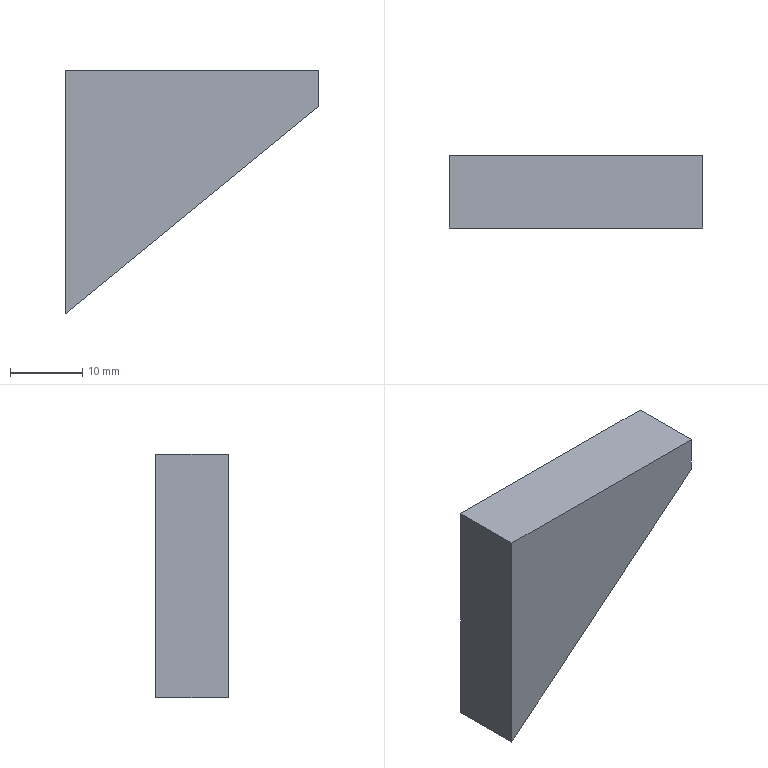Part | STEP file | Positioning_id630_x_t | 1 solid | 6 faces | box 35 x 10 x 33.636 mm | volume 6761 mm3 | plane 6
STEP:
#1=CARTESIAN_POINT('',(0.,0.,0.));
#2=DIRECTION('',(0.,0.,1.));
#3=DIRECTION('',(1.,0.,0.));
#4=AXIS2_PLACEMENT_3D('',#1,#2,#3);
#5=CARTESIAN_POINT('',(-995.002,5.,149.896));
#6=VERTEX_POINT('',#5);
#7=CARTESIAN_POINT('',(-995.002,-5.,149.896));
#8=VERTEX_POINT('',#7);
#9=CARTESIAN_POINT('',(-995.002,5.,149.896));
#10=DIRECTION('',(0.,-1.,0.));
#11=VECTOR('',#10,1.);
#12=LINE('',#9,#11);
#13=CARTESIAN_POINT('',(-960.002,2.5,178.532));
#14=DIRECTION('',(-0.6332,0.,0.774));
#15=DIRECTION('',(0.774,0.,0.6332));
#16=AXIS2_PLACEMENT_3D('',#13,#14,#15);
#17=PLANE('',#16);
#18=CARTESIAN_POINT('',(-45.222,2.5));
#19=DIRECTION('',(0.,-1.));
#20=VECTOR('',#19,1.);
#21=LINE('',#18,#20);
#22=(GEOMETRIC_REPRESENTATION_CONTEXT(2)PARAMETRIC_REPRESENTATION_CONTEXT()REPRESENTATION_CONTEXT('',''));
#23=DEFINITIONAL_REPRESENTATION('',(#21),#22);
#24=PCURVE('',#17,#23);
#25=CARTESIAN_POINT('',(-995.002,2.5,143.532));
#26=DIRECTION('',(1.,0.,0.));
#27=DIRECTION('',(0.,0.,-1.));
#28=AXIS2_PLACEMENT_3D('',#25,#26,#27);
#29=PLANE('',#28);
#30=CARTESIAN_POINT('',(-6.364,2.5));
#31=DIRECTION('',(0.,-1.));
#32=VECTOR('',#31,1.);
#33=LINE('',#30,#32);
#34=(GEOMETRIC_REPRESENTATION_CONTEXT(2)PARAMETRIC_REPRESENTATION_CONTEXT()REPRESENTATION_CONTEXT('',''));
#35=DEFINITIONAL_REPRESENTATION('',(#33),#34);
#36=PCURVE('',#29,#35);
#37=SURFACE_CURVE('',#12,(#24,#36),.PCURVE_S1.);
#38=EDGE_CURVE('',#6,#8,#37,.T.);
#39=ORIENTED_EDGE('',*,*,#38,.F.);
#40=CARTESIAN_POINT('',(-960.002,5.,178.532));
#41=VERTEX_POINT('',#40);
#42=CARTESIAN_POINT('',(-960.002,5.,178.532));
#43=DIRECTION('',(-0.774,0.,-0.6332));
#44=VECTOR('',#43,1.);
#45=LINE('',#42,#44);
#46=CARTESIAN_POINT('',(0.,2.5));
#47=DIRECTION('',(-1.,0.));
#48=VECTOR('',#47,1.);
#49=LINE('',#46,#48);
#50=(GEOMETRIC_REPRESENTATION_CONTEXT(2)PARAMETRIC_REPRESENTATION_CONTEXT()REPRESENTATION_CONTEXT('',''));
#51=DEFINITIONAL_REPRESENTATION('',(#49),#50);
#52=PCURVE('',#17,#51);
#53=CARTESIAN_POINT('',(-990.002,5.,133.532));
#54=DIRECTION('',(0.,1.,0.));
#55=DIRECTION('',(0.,0.,-1.));
#56=AXIS2_PLACEMENT_3D('',#53,#54,#55);
#57=PLANE('',#56);
#58=CARTESIAN_POINT('',(-45.,-30.));
#59=DIRECTION('',(0.6332,0.774));
#60=VECTOR('',#59,1.);
#61=LINE('',#58,#60);
#62=(GEOMETRIC_REPRESENTATION_CONTEXT(2)PARAMETRIC_REPRESENTATION_CONTEXT()REPRESENTATION_CONTEXT('',''));
#63=DEFINITIONAL_REPRESENTATION('',(#61),#62);
#64=PCURVE('',#57,#63);
#65=SURFACE_CURVE('',#45,(#52,#64),.PCURVE_S1.);
#66=EDGE_CURVE('',#41,#6,#65,.T.);
#67=ORIENTED_EDGE('',*,*,#66,.F.);
#68=CARTESIAN_POINT('',(-960.002,-5.,178.532));
#69=VERTEX_POINT('',#68);
#70=CARTESIAN_POINT('',(-960.002,-5.,178.532));
#71=DIRECTION('',(0.,1.,0.));
#72=VECTOR('',#71,1.);
#73=LINE('',#70,#72);
#74=CARTESIAN_POINT('',(0.,-7.5));
#75=DIRECTION('',(0.,1.));
#76=VECTOR('',#75,1.);
#77=LINE('',#74,#76);
#78=(GEOMETRIC_REPRESENTATION_CONTEXT(2)PARAMETRIC_REPRESENTATION_CONTEXT()REPRESENTATION_CONTEXT('',''));
#79=DEFINITIONAL_REPRESENTATION('',(#77),#78);
#80=PCURVE('',#17,#79);
#81=CARTESIAN_POINT('',(-960.002,2.5,133.532));
#82=DIRECTION('',(1.,0.,0.));
#83=DIRECTION('',(0.,0.,1.));
#84=AXIS2_PLACEMENT_3D('',#81,#82,#83);
#85=PLANE('',#84);
#86=CARTESIAN_POINT('',(45.,7.5));
#87=DIRECTION('',(0.,-1.));
#88=VECTOR('',#87,1.);
#89=LINE('',#86,#88);
#90=(GEOMETRIC_REPRESENTATION_CONTEXT(2)PARAMETRIC_REPRESENTATION_CONTEXT()REPRESENTATION_CONTEXT('',''));
#91=DEFINITIONAL_REPRESENTATION('',(#89),#90);
#92=PCURVE('',#85,#91);
#93=SURFACE_CURVE('',#73,(#80,#92),.PCURVE_S1.);
#94=EDGE_CURVE('',#69,#41,#93,.T.);
#95=ORIENTED_EDGE('',*,*,#94,.F.);
#96=CARTESIAN_POINT('',(-995.002,-5.,149.896));
#97=DIRECTION('',(0.774,0.,0.6332));
#98=VECTOR('',#97,1.);
#99=LINE('',#96,#98);
#100=CARTESIAN_POINT('',(-45.222,-7.5));
#101=DIRECTION('',(1.,0.));
#102=VECTOR('',#101,1.);
#103=LINE('',#100,#102);
#104=(GEOMETRIC_REPRESENTATION_CONTEXT(2)PARAMETRIC_REPRESENTATION_CONTEXT()REPRESENTATION_CONTEXT('',''));
#105=DEFINITIONAL_REPRESENTATION('',(#103),#104);
#106=PCURVE('',#17,#105);
#107=CARTESIAN_POINT('',(-990.002,-5.,133.532));
#108=DIRECTION('',(0.,-1.,0.));
#109=DIRECTION('',(0.,0.,1.));
#110=AXIS2_PLACEMENT_3D('',#107,#108,#109);
#111=PLANE('',#110);
#112=CARTESIAN_POINT('',(16.364,5.));
#113=DIRECTION('',(0.6332,-0.774));
#114=VECTOR('',#113,1.);
#115=LINE('',#112,#114);
#116=(GEOMETRIC_REPRESENTATION_CONTEXT(2)PARAMETRIC_REPRESENTATION_CONTEXT()REPRESENTATION_CONTEXT('',''));
#117=DEFINITIONAL_REPRESENTATION('',(#115),#116);
#118=PCURVE('',#111,#117);
#119=SURFACE_CURVE('',#99,(#106,#118),.PCURVE_S1.);
#120=EDGE_CURVE('',#8,#69,#119,.T.);
#121=ORIENTED_EDGE('',*,*,#120,.F.);
#122=EDGE_LOOP('',(#39,#67,#95,#121));
#123=FACE_BOUND('',#122,.T.);
#124=ADVANCED_FACE('',(#123),#17,.F.);
#125=CARTESIAN_POINT('',(-960.002,-5.,183.532));
#126=VERTEX_POINT('',#125);
#127=CARTESIAN_POINT('',(-960.002,-5.,178.532));
#128=DIRECTION('',(0.,0.,1.));
#129=VECTOR('',#128,1.);
#130=LINE('',#127,#129);
#131=CARTESIAN_POINT('',(45.,7.5));
#132=DIRECTION('',(1.,0.));
#133=VECTOR('',#132,1.);
#134=LINE('',#131,#133);
#135=(GEOMETRIC_REPRESENTATION_CONTEXT(2)PARAMETRIC_REPRESENTATION_CONTEXT()REPRESENTATION_CONTEXT('',''));
#136=DEFINITIONAL_REPRESENTATION('',(#134),#135);
#137=PCURVE('',#85,#136);
#138=CARTESIAN_POINT('',(45.,-30.));
#139=DIRECTION('',(1.,0.));
#140=VECTOR('',#139,1.);
#141=LINE('',#138,#140);
#142=(GEOMETRIC_REPRESENTATION_CONTEXT(2)PARAMETRIC_REPRESENTATION_CONTEXT()REPRESENTATION_CONTEXT('',''));
#143=DEFINITIONAL_REPRESENTATION('',(#141),#142);
#144=PCURVE('',#111,#143);
#145=SURFACE_CURVE('',#130,(#137,#144),.PCURVE_S1.);
#146=EDGE_CURVE('',#69,#126,#145,.T.);
#147=ORIENTED_EDGE('',*,*,#146,.F.);
#148=ORIENTED_EDGE('',*,*,#94,.T.);
#149=CARTESIAN_POINT('',(-960.002,5.,183.532));
#150=VERTEX_POINT('',#149);
#151=CARTESIAN_POINT('',(-960.002,5.,178.532));
#152=DIRECTION('',(0.,0.,1.));
#153=VECTOR('',#152,1.);
#154=LINE('',#151,#153);
#155=CARTESIAN_POINT('',(45.,-2.5));
#156=DIRECTION('',(1.,0.));
#157=VECTOR('',#156,1.);
#158=LINE('',#155,#157);
#159=(GEOMETRIC_REPRESENTATION_CONTEXT(2)PARAMETRIC_REPRESENTATION_CONTEXT()REPRESENTATION_CONTEXT('',''));
#160=DEFINITIONAL_REPRESENTATION('',(#158),#159);
#161=PCURVE('',#85,#160);
#162=CARTESIAN_POINT('',(-45.,-30.));
#163=DIRECTION('',(-1.,0.));
#164=VECTOR('',#163,1.);
#165=LINE('',#162,#164);
#166=(GEOMETRIC_REPRESENTATION_CONTEXT(2)PARAMETRIC_REPRESENTATION_CONTEXT()REPRESENTATION_CONTEXT('',''));
#167=DEFINITIONAL_REPRESENTATION('',(#165),#166);
#168=PCURVE('',#57,#167);
#169=SURFACE_CURVE('',#154,(#161,#168),.PCURVE_S1.);
#170=EDGE_CURVE('',#41,#150,#169,.T.);
#171=ORIENTED_EDGE('',*,*,#170,.T.);
#172=CARTESIAN_POINT('',(-960.002,5.,183.532));
#173=DIRECTION('',(0.,-1.,0.));
#174=VECTOR('',#173,1.);
#175=LINE('',#172,#174);
#176=CARTESIAN_POINT('',(50.,-2.5));
#177=DIRECTION('',(0.,1.));
#178=VECTOR('',#177,1.);
#179=LINE('',#176,#178);
#180=(GEOMETRIC_REPRESENTATION_CONTEXT(2)PARAMETRIC_REPRESENTATION_CONTEXT()REPRESENTATION_CONTEXT('',''));
#181=DEFINITIONAL_REPRESENTATION('',(#179),#180);
#182=PCURVE('',#85,#181);
#183=CARTESIAN_POINT('',(-990.002,2.5,183.532));
#184=DIRECTION('',(0.,0.,1.));
#185=DIRECTION('',(-1.,0.,0.));
#186=AXIS2_PLACEMENT_3D('',#183,#184,#185);
#187=PLANE('',#186);
#188=CARTESIAN_POINT('',(-30.,-2.5));
#189=DIRECTION('',(0.,1.));
#190=VECTOR('',#189,1.);
#191=LINE('',#188,#190);
#192=(GEOMETRIC_REPRESENTATION_CONTEXT(2)PARAMETRIC_REPRESENTATION_CONTEXT()REPRESENTATION_CONTEXT('',''));
#193=DEFINITIONAL_REPRESENTATION('',(#191),#192);
#194=PCURVE('',#187,#193);
#195=SURFACE_CURVE('',#175,(#182,#194),.PCURVE_S1.);
#196=EDGE_CURVE('',#150,#126,#195,.T.);
#197=ORIENTED_EDGE('',*,*,#196,.T.);
#198=EDGE_LOOP('',(#147,#148,#171,#197));
#199=FACE_BOUND('',#198,.T.);
#200=ADVANCED_FACE('',(#199),#85,.T.);
#201=CARTESIAN_POINT('',(-995.002,5.,183.532));
#202=VERTEX_POINT('',#201);
#203=CARTESIAN_POINT('',(-995.002,5.,183.532));
#204=DIRECTION('',(0.,0.,-1.));
#205=VECTOR('',#204,1.);
#206=LINE('',#203,#205);
#207=CARTESIAN_POINT('',(-50.,5.));
#208=DIRECTION('',(1.,0.));
#209=VECTOR('',#208,1.);
#210=LINE('',#207,#209);
#211=(GEOMETRIC_REPRESENTATION_CONTEXT(2)PARAMETRIC_REPRESENTATION_CONTEXT()REPRESENTATION_CONTEXT('',''));
#212=DEFINITIONAL_REPRESENTATION('',(#210),#211);
#213=PCURVE('',#57,#212);
#214=CARTESIAN_POINT('',(-40.,2.5));
#215=DIRECTION('',(1.,0.));
#216=VECTOR('',#215,1.);
#217=LINE('',#214,#216);
#218=(GEOMETRIC_REPRESENTATION_CONTEXT(2)PARAMETRIC_REPRESENTATION_CONTEXT()REPRESENTATION_CONTEXT('',''));
#219=DEFINITIONAL_REPRESENTATION('',(#217),#218);
#220=PCURVE('',#29,#219);
#221=SURFACE_CURVE('',#206,(#213,#220),.PCURVE_S1.);
#222=EDGE_CURVE('',#202,#6,#221,.T.);
#223=ORIENTED_EDGE('',*,*,#222,.F.);
#224=CARTESIAN_POINT('',(-995.002,5.,183.532));
#225=DIRECTION('',(1.,0.,0.));
#226=VECTOR('',#225,1.);
#227=LINE('',#224,#226);
#228=CARTESIAN_POINT('',(-50.,5.));
#229=DIRECTION('',(0.,-1.));
#230=VECTOR('',#229,1.);
#231=LINE('',#228,#230);
#232=(GEOMETRIC_REPRESENTATION_CONTEXT(2)PARAMETRIC_REPRESENTATION_CONTEXT()REPRESENTATION_CONTEXT('',''));
#233=DEFINITIONAL_REPRESENTATION('',(#231),#232);
#234=PCURVE('',#57,#233);
#235=CARTESIAN_POINT('',(5.,-2.5));
#236=DIRECTION('',(-1.,0.));
#237=VECTOR('',#236,1.);
#238=LINE('',#235,#237);
#239=(GEOMETRIC_REPRESENTATION_CONTEXT(2)PARAMETRIC_REPRESENTATION_CONTEXT()REPRESENTATION_CONTEXT('',''));
#240=DEFINITIONAL_REPRESENTATION('',(#238),#239);
#241=PCURVE('',#187,#240);
#242=SURFACE_CURVE('',#227,(#234,#241),.PCURVE_S1.);
#243=EDGE_CURVE('',#202,#150,#242,.T.);
#244=ORIENTED_EDGE('',*,*,#243,.T.);
#245=ORIENTED_EDGE('',*,*,#170,.F.);
#246=ORIENTED_EDGE('',*,*,#66,.T.);
#247=EDGE_LOOP('',(#223,#244,#245,#246));
#248=FACE_BOUND('',#247,.T.);
#249=ADVANCED_FACE('',(#248),#57,.T.);
#250=CARTESIAN_POINT('',(-995.002,-5.,183.532));
#251=VERTEX_POINT('',#250);
#252=CARTESIAN_POINT('',(-995.002,-5.,149.896));
#253=DIRECTION('',(0.,0.,1.));
#254=VECTOR('',#253,1.);
#255=LINE('',#252,#254);
#256=CARTESIAN_POINT('',(16.364,5.));
#257=DIRECTION('',(1.,0.));
#258=VECTOR('',#257,1.);
#259=LINE('',#256,#258);
#260=(GEOMETRIC_REPRESENTATION_CONTEXT(2)PARAMETRIC_REPRESENTATION_CONTEXT()REPRESENTATION_CONTEXT('',''));
#261=DEFINITIONAL_REPRESENTATION('',(#259),#260);
#262=PCURVE('',#111,#261);
#263=CARTESIAN_POINT('',(-6.364,-7.5));
#264=DIRECTION('',(-1.,0.));
#265=VECTOR('',#264,1.);
#266=LINE('',#263,#265);
#267=(GEOMETRIC_REPRESENTATION_CONTEXT(2)PARAMETRIC_REPRESENTATION_CONTEXT()REPRESENTATION_CONTEXT('',''));
#268=DEFINITIONAL_REPRESENTATION('',(#266),#267);
#269=PCURVE('',#29,#268);
#270=SURFACE_CURVE('',#255,(#262,#269),.PCURVE_S1.);
#271=EDGE_CURVE('',#8,#251,#270,.T.);
#272=ORIENTED_EDGE('',*,*,#271,.F.);
#273=ORIENTED_EDGE('',*,*,#120,.T.);
#274=ORIENTED_EDGE('',*,*,#146,.T.);
#275=CARTESIAN_POINT('',(-960.002,-5.,183.532));
#276=DIRECTION('',(-1.,0.,0.));
#277=VECTOR('',#276,1.);
#278=LINE('',#275,#277);
#279=CARTESIAN_POINT('',(50.,-30.));
#280=DIRECTION('',(0.,1.));
#281=VECTOR('',#280,1.);
#282=LINE('',#279,#281);
#283=(GEOMETRIC_REPRESENTATION_CONTEXT(2)PARAMETRIC_REPRESENTATION_CONTEXT()REPRESENTATION_CONTEXT('',''));
#284=DEFINITIONAL_REPRESENTATION('',(#282),#283);
#285=PCURVE('',#111,#284);
#286=CARTESIAN_POINT('',(-30.,7.5));
#287=DIRECTION('',(1.,0.));
#288=VECTOR('',#287,1.);
#289=LINE('',#286,#288);
#290=(GEOMETRIC_REPRESENTATION_CONTEXT(2)PARAMETRIC_REPRESENTATION_CONTEXT()REPRESENTATION_CONTEXT('',''));
#291=DEFINITIONAL_REPRESENTATION('',(#289),#290);
#292=PCURVE('',#187,#291);
#293=SURFACE_CURVE('',#278,(#285,#292),.PCURVE_S1.);
#294=EDGE_CURVE('',#126,#251,#293,.T.);
#295=ORIENTED_EDGE('',*,*,#294,.T.);
#296=EDGE_LOOP('',(#272,#273,#274,#295));
#297=FACE_BOUND('',#296,.T.);
#298=ADVANCED_FACE('',(#297),#111,.T.);
#299=CARTESIAN_POINT('',(-995.002,-5.,183.532));
#300=DIRECTION('',(0.,1.,0.));
#301=VECTOR('',#300,1.);
#302=LINE('',#299,#301);
#303=CARTESIAN_POINT('',(5.,7.5));
#304=DIRECTION('',(0.,-1.));
#305=VECTOR('',#304,1.);
#306=LINE('',#303,#305);
#307=(GEOMETRIC_REPRESENTATION_CONTEXT(2)PARAMETRIC_REPRESENTATION_CONTEXT()REPRESENTATION_CONTEXT('',''));
#308=DEFINITIONAL_REPRESENTATION('',(#306),#307);
#309=PCURVE('',#187,#308);
#310=CARTESIAN_POINT('',(-40.,-7.5));
#311=DIRECTION('',(0.,1.));
#312=VECTOR('',#311,1.);
#313=LINE('',#310,#312);
#314=(GEOMETRIC_REPRESENTATION_CONTEXT(2)PARAMETRIC_REPRESENTATION_CONTEXT()REPRESENTATION_CONTEXT('',''));
#315=DEFINITIONAL_REPRESENTATION('',(#313),#314);
#316=PCURVE('',#29,#315);
#317=SURFACE_CURVE('',#302,(#309,#316),.PCURVE_S1.);
#318=EDGE_CURVE('',#251,#202,#317,.T.);
#319=ORIENTED_EDGE('',*,*,#318,.F.);
#320=ORIENTED_EDGE('',*,*,#294,.F.);
#321=ORIENTED_EDGE('',*,*,#196,.F.);
#322=ORIENTED_EDGE('',*,*,#243,.F.);
#323=EDGE_LOOP('',(#319,#320,#321,#322));
#324=FACE_BOUND('',#323,.T.);
#325=ADVANCED_FACE('',(#324),#187,.T.);
#326=ORIENTED_EDGE('',*,*,#271,.T.);
#327=ORIENTED_EDGE('',*,*,#318,.T.);
#328=ORIENTED_EDGE('',*,*,#222,.T.);
#329=ORIENTED_EDGE('',*,*,#38,.T.);
#330=EDGE_LOOP('',(#326,#327,#328,#329));
#331=FACE_BOUND('',#330,.T.);
#332=ADVANCED_FACE('',(#331),#29,.F.);
#333=CLOSED_SHELL('',(#124,#200,#249,#298,#325,#332));
#334=MANIFOLD_SOLID_BREP('',#333);
#335=(LENGTH_UNIT()NAMED_UNIT(*)SI_UNIT(.MILLI.,.METRE.));
#336=UNCERTAINTY_MEASURE_WITH_UNIT(LENGTH_MEASURE(0.0000001),#335,'','');
#337=(NAMED_UNIT(*)PLANE_ANGLE_UNIT()SI_UNIT($,.RADIAN.));
#338=(NAMED_UNIT(*)SI_UNIT($,.STERADIAN.)SOLID_ANGLE_UNIT());
#339=(GEOMETRIC_REPRESENTATION_CONTEXT(3)GLOBAL_UNCERTAINTY_ASSIGNED_CONTEXT((#336))GLOBAL_UNIT_ASSIGNED_CONTEXT((#335,#337,#338))REPRESENTATION_CONTEXT('',''));
#340=ADVANCED_BREP_SHAPE_REPRESENTATION('',(#4,#334),#339);